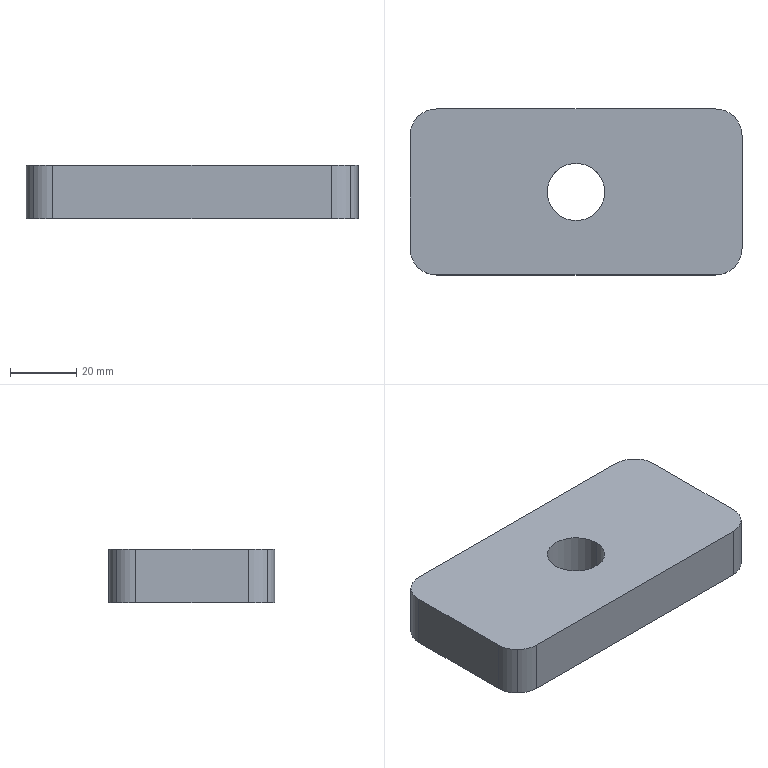Part | STEP file | DCV-000-025 | 1 solid | 16 faces | box 100 x 50 x 16 mm | volume 75363 mm3 | cylinder 10 | plane 6 | commonest cylinder face diameters 16 x8 17.294 x2
STEP:
#1=CARTESIAN_POINT('',(0.,0.,0.));
#2=DIRECTION('',(0.,0.,1.));
#3=DIRECTION('',(1.,0.,0.));
#4=AXIS2_PLACEMENT_3D('',#1,#2,#3);
#5=CARTESIAN_POINT('',(-50.,-17.,0.));
#6=VERTEX_POINT('',#5);
#7=CARTESIAN_POINT('',(-47.657,-22.657,0.));
#8=VERTEX_POINT('',#7);
#9=CARTESIAN_POINT('',(-42.,-17.,0.));
#10=DIRECTION('',(0.,0.,1.));
#11=DIRECTION('',(-0.7071,-0.7071,0.));
#12=AXIS2_PLACEMENT_3D('',#9,#10,#11);
#13=CIRCLE('',#12,8.);
#14=CARTESIAN_POINT('',(-42.,-17.,0.));
#15=DIRECTION('',(0.,0.,1.));
#16=DIRECTION('',(-0.7071,-0.7071,0.));
#17=AXIS2_PLACEMENT_3D('',#14,#15,#16);
#18=CYLINDRICAL_SURFACE('',#17,8.);
#19=CARTESIAN_POINT('',(0.,0.));
#20=DIRECTION('',(1.,0.));
#21=VECTOR('',#20,1.);
#22=LINE('',#19,#21);
#23=(GEOMETRIC_REPRESENTATION_CONTEXT(2)PARAMETRIC_REPRESENTATION_CONTEXT()REPRESENTATION_CONTEXT('',''));
#24=DEFINITIONAL_REPRESENTATION('',(#22),#23);
#25=PCURVE('',#18,#24);
#26=CARTESIAN_POINT('',(0.,0.,0.));
#27=DIRECTION('',(0.,0.,1.));
#28=DIRECTION('',(1.,0.,0.));
#29=AXIS2_PLACEMENT_3D('',#26,#27,#28);
#30=PLANE('',#29);
#31=CARTESIAN_POINT('',(-42.,-17.));
#32=DIRECTION('',(-0.7071,-0.7071));
#33=AXIS2_PLACEMENT_2D('',#31,#32);
#34=CIRCLE('',#33,8.);
#35=(GEOMETRIC_REPRESENTATION_CONTEXT(2)PARAMETRIC_REPRESENTATION_CONTEXT()REPRESENTATION_CONTEXT('',''));
#36=DEFINITIONAL_REPRESENTATION('',(#34),#35);
#37=PCURVE('',#30,#36);
#38=SURFACE_CURVE('',#13,(#25,#37),.PCURVE_S1.);
#39=EDGE_CURVE('',#6,#8,#38,.T.);
#40=ORIENTED_EDGE('',*,*,#39,.T.);
#41=CARTESIAN_POINT('',(-47.657,-22.657,16.));
#42=VERTEX_POINT('',#41);
#43=CARTESIAN_POINT('',(-47.657,-22.657,0.));
#44=DIRECTION('',(0.,0.,1.));
#45=VECTOR('',#44,1.);
#46=LINE('',#43,#45);
#47=CARTESIAN_POINT('',(6.283,0.));
#48=DIRECTION('',(0.,1.));
#49=VECTOR('',#48,1.);
#50=LINE('',#47,#49);
#51=(GEOMETRIC_REPRESENTATION_CONTEXT(2)PARAMETRIC_REPRESENTATION_CONTEXT()REPRESENTATION_CONTEXT('',''));
#52=DEFINITIONAL_REPRESENTATION('',(#50),#51);
#53=PCURVE('',#18,#52);
#54=CARTESIAN_POINT('',(-42.,-17.,0.));
#55=DIRECTION('',(0.,0.,1.));
#56=DIRECTION('',(-0.7071,-0.7071,0.));
#57=AXIS2_PLACEMENT_3D('',#54,#55,#56);
#58=CYLINDRICAL_SURFACE('',#57,8.);
#59=CARTESIAN_POINT('',(0.,0.));
#60=DIRECTION('',(0.,1.));
#61=VECTOR('',#60,1.);
#62=LINE('',#59,#61);
#63=(GEOMETRIC_REPRESENTATION_CONTEXT(2)PARAMETRIC_REPRESENTATION_CONTEXT()REPRESENTATION_CONTEXT('',''));
#64=DEFINITIONAL_REPRESENTATION('',(#62),#63);
#65=PCURVE('',#58,#64);
#66=SURFACE_CURVE('',#46,(#53,#65),.PCURVE_S1.);
#67=EDGE_CURVE('',#8,#42,#66,.T.);
#68=ORIENTED_EDGE('',*,*,#67,.T.);
#69=CARTESIAN_POINT('',(-50.,-17.,16.));
#70=VERTEX_POINT('',#69);
#71=CARTESIAN_POINT('',(-42.,-17.,16.));
#72=DIRECTION('',(0.,0.,-1.));
#73=DIRECTION('',(-0.7071,-0.7071,0.));
#74=AXIS2_PLACEMENT_3D('',#71,#72,#73);
#75=CIRCLE('',#74,8.);
#76=CARTESIAN_POINT('',(6.283,16.));
#77=DIRECTION('',(-1.,0.));
#78=VECTOR('',#77,1.);
#79=LINE('',#76,#78);
#80=(GEOMETRIC_REPRESENTATION_CONTEXT(2)PARAMETRIC_REPRESENTATION_CONTEXT()REPRESENTATION_CONTEXT('',''));
#81=DEFINITIONAL_REPRESENTATION('',(#79),#80);
#82=PCURVE('',#18,#81);
#83=CARTESIAN_POINT('',(0.,0.,16.));
#84=DIRECTION('',(0.,0.,1.));
#85=DIRECTION('',(1.,0.,0.));
#86=AXIS2_PLACEMENT_3D('',#83,#84,#85);
#87=PLANE('',#86);
#88=CARTESIAN_POINT('',(-47.657,-22.657));
#89=CARTESIAN_POINT('',(-57.455,-12.859));
#90=CARTESIAN_POINT('',(-44.071,-9.273));
#91=CARTESIAN_POINT('',(-30.686,-5.686));
#92=CARTESIAN_POINT('',(-34.273,-19.071));
#93=CARTESIAN_POINT('',(-37.859,-32.455));
#94=CARTESIAN_POINT('',(-47.657,-22.657));
#95=(BOUNDED_CURVE()B_SPLINE_CURVE(2,(#88,#89,#90,#91,#92,#93,#94),.UNSPECIFIED.,.T.,.F.)B_SPLINE_CURVE_WITH_KNOTS((1,2,2,2,2,1),(-2.094,0.,2.094,4.189,6.283,8.378),.UNSPECIFIED.)CURVE()GEOMETRIC_REPRESENTATION_ITEM()RATIONAL_B_SPLINE_CURVE((1.,0.5,1.,0.5,1.,0.5,1.))REPRESENTATION_ITEM(''));
#96=(GEOMETRIC_REPRESENTATION_CONTEXT(2)PARAMETRIC_REPRESENTATION_CONTEXT()REPRESENTATION_CONTEXT('',''));
#97=DEFINITIONAL_REPRESENTATION('',(#95),#96);
#98=PCURVE('',#87,#97);
#99=SURFACE_CURVE('',#75,(#82,#98),.PCURVE_S1.);
#100=EDGE_CURVE('',#42,#70,#99,.T.);
#101=ORIENTED_EDGE('',*,*,#100,.T.);
#102=CARTESIAN_POINT('',(-50.,-17.,0.));
#103=DIRECTION('',(0.,0.,-1.));
#104=VECTOR('',#103,1.);
#105=LINE('',#102,#104);
#106=CARTESIAN_POINT('',(5.498,0.));
#107=DIRECTION('',(0.,-1.));
#108=VECTOR('',#107,1.);
#109=LINE('',#106,#108);
#110=(GEOMETRIC_REPRESENTATION_CONTEXT(2)PARAMETRIC_REPRESENTATION_CONTEXT()REPRESENTATION_CONTEXT('',''));
#111=DEFINITIONAL_REPRESENTATION('',(#109),#110);
#112=PCURVE('',#18,#111);
#113=CARTESIAN_POINT('',(-50.,25.,0.));
#114=DIRECTION('',(-1.,0.,0.));
#115=DIRECTION('',(0.,0.,1.));
#116=AXIS2_PLACEMENT_3D('',#113,#114,#115);
#117=PLANE('',#116);
#118=CARTESIAN_POINT('',(0.,-42.));
#119=DIRECTION('',(-1.,0.));
#120=VECTOR('',#119,1.);
#121=LINE('',#118,#120);
#122=(GEOMETRIC_REPRESENTATION_CONTEXT(2)PARAMETRIC_REPRESENTATION_CONTEXT()REPRESENTATION_CONTEXT('',''));
#123=DEFINITIONAL_REPRESENTATION('',(#121),#122);
#124=PCURVE('',#117,#123);
#125=SURFACE_CURVE('',#105,(#112,#124),.PCURVE_S1.);
#126=EDGE_CURVE('',#70,#6,#125,.T.);
#127=ORIENTED_EDGE('',*,*,#126,.T.);
#128=EDGE_LOOP('',(#40,#68,#101,#127));
#129=FACE_BOUND('',#128,.T.);
#130=ADVANCED_FACE('',(#129),#18,.T.);
#131=CARTESIAN_POINT('',(42.,-25.,0.));
#132=VERTEX_POINT('',#131);
#133=CARTESIAN_POINT('',(47.657,-22.657,0.));
#134=VERTEX_POINT('',#133);
#135=CARTESIAN_POINT('',(42.,-17.,0.));
#136=DIRECTION('',(0.,0.,1.));
#137=DIRECTION('',(0.7071,-0.7071,0.));
#138=AXIS2_PLACEMENT_3D('',#135,#136,#137);
#139=CIRCLE('',#138,8.);
#140=CARTESIAN_POINT('',(42.,-17.,0.));
#141=DIRECTION('',(0.,0.,1.));
#142=DIRECTION('',(0.7071,-0.7071,0.));
#143=AXIS2_PLACEMENT_3D('',#140,#141,#142);
#144=CYLINDRICAL_SURFACE('',#143,8.);
#145=CARTESIAN_POINT('',(0.,0.));
#146=DIRECTION('',(1.,0.));
#147=VECTOR('',#146,1.);
#148=LINE('',#145,#147);
#149=(GEOMETRIC_REPRESENTATION_CONTEXT(2)PARAMETRIC_REPRESENTATION_CONTEXT()REPRESENTATION_CONTEXT('',''));
#150=DEFINITIONAL_REPRESENTATION('',(#148),#149);
#151=PCURVE('',#144,#150);
#152=CARTESIAN_POINT('',(42.,-17.));
#153=DIRECTION('',(0.7071,-0.7071));
#154=AXIS2_PLACEMENT_2D('',#152,#153);
#155=CIRCLE('',#154,8.);
#156=(GEOMETRIC_REPRESENTATION_CONTEXT(2)PARAMETRIC_REPRESENTATION_CONTEXT()REPRESENTATION_CONTEXT('',''));
#157=DEFINITIONAL_REPRESENTATION('',(#155),#156);
#158=PCURVE('',#30,#157);
#159=SURFACE_CURVE('',#139,(#151,#158),.PCURVE_S1.);
#160=EDGE_CURVE('',#132,#134,#159,.T.);
#161=ORIENTED_EDGE('',*,*,#160,.T.);
#162=CARTESIAN_POINT('',(47.657,-22.657,16.));
#163=VERTEX_POINT('',#162);
#164=CARTESIAN_POINT('',(47.657,-22.657,0.));
#165=DIRECTION('',(0.,0.,1.));
#166=VECTOR('',#165,1.);
#167=LINE('',#164,#166);
#168=CARTESIAN_POINT('',(6.283,0.));
#169=DIRECTION('',(0.,1.));
#170=VECTOR('',#169,1.);
#171=LINE('',#168,#170);
#172=(GEOMETRIC_REPRESENTATION_CONTEXT(2)PARAMETRIC_REPRESENTATION_CONTEXT()REPRESENTATION_CONTEXT('',''));
#173=DEFINITIONAL_REPRESENTATION('',(#171),#172);
#174=PCURVE('',#144,#173);
#175=CARTESIAN_POINT('',(42.,-17.,0.));
#176=DIRECTION('',(0.,0.,1.));
#177=DIRECTION('',(0.7071,-0.7071,0.));
#178=AXIS2_PLACEMENT_3D('',#175,#176,#177);
#179=CYLINDRICAL_SURFACE('',#178,8.);
#180=CARTESIAN_POINT('',(0.,0.));
#181=DIRECTION('',(0.,1.));
#182=VECTOR('',#181,1.);
#183=LINE('',#180,#182);
#184=(GEOMETRIC_REPRESENTATION_CONTEXT(2)PARAMETRIC_REPRESENTATION_CONTEXT()REPRESENTATION_CONTEXT('',''));
#185=DEFINITIONAL_REPRESENTATION('',(#183),#184);
#186=PCURVE('',#179,#185);
#187=SURFACE_CURVE('',#167,(#174,#186),.PCURVE_S1.);
#188=EDGE_CURVE('',#134,#163,#187,.T.);
#189=ORIENTED_EDGE('',*,*,#188,.T.);
#190=CARTESIAN_POINT('',(42.,-25.,16.));
#191=VERTEX_POINT('',#190);
#192=CARTESIAN_POINT('',(42.,-17.,16.));
#193=DIRECTION('',(0.,0.,-1.));
#194=DIRECTION('',(0.7071,-0.7071,0.));
#195=AXIS2_PLACEMENT_3D('',#192,#193,#194);
#196=CIRCLE('',#195,8.);
#197=CARTESIAN_POINT('',(6.283,16.));
#198=DIRECTION('',(-1.,0.));
#199=VECTOR('',#198,1.);
#200=LINE('',#197,#199);
#201=(GEOMETRIC_REPRESENTATION_CONTEXT(2)PARAMETRIC_REPRESENTATION_CONTEXT()REPRESENTATION_CONTEXT('',''));
#202=DEFINITIONAL_REPRESENTATION('',(#200),#201);
#203=PCURVE('',#144,#202);
#204=CARTESIAN_POINT('',(47.657,-22.657));
#205=CARTESIAN_POINT('',(37.859,-32.455));
#206=CARTESIAN_POINT('',(34.273,-19.071));
#207=CARTESIAN_POINT('',(30.686,-5.686));
#208=CARTESIAN_POINT('',(44.071,-9.273));
#209=CARTESIAN_POINT('',(57.455,-12.859));
#210=CARTESIAN_POINT('',(47.657,-22.657));
#211=(BOUNDED_CURVE()B_SPLINE_CURVE(2,(#204,#205,#206,#207,#208,#209,#210),.UNSPECIFIED.,.T.,.F.)B_SPLINE_CURVE_WITH_KNOTS((1,2,2,2,2,1),(-2.094,0.,2.094,4.189,6.283,8.378),.UNSPECIFIED.)CURVE()GEOMETRIC_REPRESENTATION_ITEM()RATIONAL_B_SPLINE_CURVE((1.,0.5,1.,0.5,1.,0.5,1.))REPRESENTATION_ITEM(''));
#212=(GEOMETRIC_REPRESENTATION_CONTEXT(2)PARAMETRIC_REPRESENTATION_CONTEXT()REPRESENTATION_CONTEXT('',''));
#213=DEFINITIONAL_REPRESENTATION('',(#211),#212);
#214=PCURVE('',#87,#213);
#215=SURFACE_CURVE('',#196,(#203,#214),.PCURVE_S1.);
#216=EDGE_CURVE('',#163,#191,#215,.T.);
#217=ORIENTED_EDGE('',*,*,#216,.T.);
#218=CARTESIAN_POINT('',(42.,-25.,0.));
#219=DIRECTION('',(0.,0.,-1.));
#220=VECTOR('',#219,1.);
#221=LINE('',#218,#220);
#222=CARTESIAN_POINT('',(5.498,0.));
#223=DIRECTION('',(0.,-1.));
#224=VECTOR('',#223,1.);
#225=LINE('',#222,#224);
#226=(GEOMETRIC_REPRESENTATION_CONTEXT(2)PARAMETRIC_REPRESENTATION_CONTEXT()REPRESENTATION_CONTEXT('',''));
#227=DEFINITIONAL_REPRESENTATION('',(#225),#226);
#228=PCURVE('',#144,#227);
#229=CARTESIAN_POINT('',(-50.,-25.,0.));
#230=DIRECTION('',(0.,-1.,0.));
#231=DIRECTION('',(0.,0.,-1.));
#232=AXIS2_PLACEMENT_3D('',#229,#230,#231);
#233=PLANE('',#232);
#234=CARTESIAN_POINT('',(0.,92.));
#235=DIRECTION('',(1.,0.));
#236=VECTOR('',#235,1.);
#237=LINE('',#234,#236);
#238=(GEOMETRIC_REPRESENTATION_CONTEXT(2)PARAMETRIC_REPRESENTATION_CONTEXT()REPRESENTATION_CONTEXT('',''));
#239=DEFINITIONAL_REPRESENTATION('',(#237),#238);
#240=PCURVE('',#233,#239);
#241=SURFACE_CURVE('',#221,(#228,#240),.PCURVE_S1.);
#242=EDGE_CURVE('',#191,#132,#241,.T.);
#243=ORIENTED_EDGE('',*,*,#242,.T.);
#244=EDGE_LOOP('',(#161,#189,#217,#243));
#245=FACE_BOUND('',#244,.T.);
#246=ADVANCED_FACE('',(#245),#144,.T.);
#247=CARTESIAN_POINT('',(50.,17.,0.));
#248=VERTEX_POINT('',#247);
#249=CARTESIAN_POINT('',(47.657,22.657,0.));
#250=VERTEX_POINT('',#249);
#251=CARTESIAN_POINT('',(42.,17.,0.));
#252=DIRECTION('',(0.,0.,1.));
#253=DIRECTION('',(0.7071,0.7071,0.));
#254=AXIS2_PLACEMENT_3D('',#251,#252,#253);
#255=CIRCLE('',#254,8.);
#256=CARTESIAN_POINT('',(42.,17.,0.));
#257=DIRECTION('',(0.,0.,1.));
#258=DIRECTION('',(0.7071,0.7071,0.));
#259=AXIS2_PLACEMENT_3D('',#256,#257,#258);
#260=CYLINDRICAL_SURFACE('',#259,8.);
#261=CARTESIAN_POINT('',(0.,0.));
#262=DIRECTION('',(1.,0.));
#263=VECTOR('',#262,1.);
#264=LINE('',#261,#263);
#265=(GEOMETRIC_REPRESENTATION_CONTEXT(2)PARAMETRIC_REPRESENTATION_CONTEXT()REPRESENTATION_CONTEXT('',''));
#266=DEFINITIONAL_REPRESENTATION('',(#264),#265);
#267=PCURVE('',#260,#266);
#268=CARTESIAN_POINT('',(42.,17.));
#269=DIRECTION('',(0.7071,0.7071));
#270=AXIS2_PLACEMENT_2D('',#268,#269);
#271=CIRCLE('',#270,8.);
#272=(GEOMETRIC_REPRESENTATION_CONTEXT(2)PARAMETRIC_REPRESENTATION_CONTEXT()REPRESENTATION_CONTEXT('',''));
#273=DEFINITIONAL_REPRESENTATION('',(#271),#272);
#274=PCURVE('',#30,#273);
#275=SURFACE_CURVE('',#255,(#267,#274),.PCURVE_S1.);
#276=EDGE_CURVE('',#248,#250,#275,.T.);
#277=ORIENTED_EDGE('',*,*,#276,.T.);
#278=CARTESIAN_POINT('',(47.657,22.657,16.));
#279=VERTEX_POINT('',#278);
#280=CARTESIAN_POINT('',(47.657,22.657,0.));
#281=DIRECTION('',(0.,0.,1.));
#282=VECTOR('',#281,1.);
#283=LINE('',#280,#282);
#284=CARTESIAN_POINT('',(6.283,0.));
#285=DIRECTION('',(0.,1.));
#286=VECTOR('',#285,1.);
#287=LINE('',#284,#286);
#288=(GEOMETRIC_REPRESENTATION_CONTEXT(2)PARAMETRIC_REPRESENTATION_CONTEXT()REPRESENTATION_CONTEXT('',''));
#289=DEFINITIONAL_REPRESENTATION('',(#287),#288);
#290=PCURVE('',#260,#289);
#291=CARTESIAN_POINT('',(42.,17.,0.));
#292=DIRECTION('',(0.,0.,1.));
#293=DIRECTION('',(0.7071,0.7071,0.));
#294=AXIS2_PLACEMENT_3D('',#291,#292,#293);
#295=CYLINDRICAL_SURFACE('',#294,8.);
#296=CARTESIAN_POINT('',(0.,0.));
#297=DIRECTION('',(0.,1.));
#298=VECTOR('',#297,1.);
#299=LINE('',#296,#298);
#300=(GEOMETRIC_REPRESENTATION_CONTEXT(2)PARAMETRIC_REPRESENTATION_CONTEXT()REPRESENTATION_CONTEXT('',''));
#301=DEFINITIONAL_REPRESENTATION('',(#299),#300);
#302=PCURVE('',#295,#301);
#303=SURFACE_CURVE('',#283,(#290,#302),.PCURVE_S1.);
#304=EDGE_CURVE('',#250,#279,#303,.T.);
#305=ORIENTED_EDGE('',*,*,#304,.T.);
#306=CARTESIAN_POINT('',(50.,17.,16.));
#307=VERTEX_POINT('',#306);
#308=CARTESIAN_POINT('',(42.,17.,16.));
#309=DIRECTION('',(0.,0.,-1.));
#310=DIRECTION('',(0.7071,0.7071,0.));
#311=AXIS2_PLACEMENT_3D('',#308,#309,#310);
#312=CIRCLE('',#311,8.);
#313=CARTESIAN_POINT('',(6.283,16.));
#314=DIRECTION('',(-1.,0.));
#315=VECTOR('',#314,1.);
#316=LINE('',#313,#315);
#317=(GEOMETRIC_REPRESENTATION_CONTEXT(2)PARAMETRIC_REPRESENTATION_CONTEXT()REPRESENTATION_CONTEXT('',''));
#318=DEFINITIONAL_REPRESENTATION('',(#316),#317);
#319=PCURVE('',#260,#318);
#320=CARTESIAN_POINT('',(47.657,22.657));
#321=CARTESIAN_POINT('',(57.455,12.859));
#322=CARTESIAN_POINT('',(44.071,9.273));
#323=CARTESIAN_POINT('',(30.686,5.686));
#324=CARTESIAN_POINT('',(34.273,19.071));
#325=CARTESIAN_POINT('',(37.859,32.455));
#326=CARTESIAN_POINT('',(47.657,22.657));
#327=(BOUNDED_CURVE()B_SPLINE_CURVE(2,(#320,#321,#322,#323,#324,#325,#326),.UNSPECIFIED.,.T.,.F.)B_SPLINE_CURVE_WITH_KNOTS((1,2,2,2,2,1),(-2.094,0.,2.094,4.189,6.283,8.378),.UNSPECIFIED.)CURVE()GEOMETRIC_REPRESENTATION_ITEM()RATIONAL_B_SPLINE_CURVE((1.,0.5,1.,0.5,1.,0.5,1.))REPRESENTATION_ITEM(''));
#328=(GEOMETRIC_REPRESENTATION_CONTEXT(2)PARAMETRIC_REPRESENTATION_CONTEXT()REPRESENTATION_CONTEXT('',''));
#329=DEFINITIONAL_REPRESENTATION('',(#327),#328);
#330=PCURVE('',#87,#329);
#331=SURFACE_CURVE('',#312,(#319,#330),.PCURVE_S1.);
#332=EDGE_CURVE('',#279,#307,#331,.T.);
#333=ORIENTED_EDGE('',*,*,#332,.T.);
#334=CARTESIAN_POINT('',(50.,17.,0.));
#335=DIRECTION('',(0.,0.,-1.));
#336=VECTOR('',#335,1.);
#337=LINE('',#334,#336);
#338=CARTESIAN_POINT('',(5.498,0.));
#339=DIRECTION('',(0.,-1.));
#340=VECTOR('',#339,1.);
#341=LINE('',#338,#340);
#342=(GEOMETRIC_REPRESENTATION_CONTEXT(2)PARAMETRIC_REPRESENTATION_CONTEXT()REPRESENTATION_CONTEXT('',''));
#343=DEFINITIONAL_REPRESENTATION('',(#341),#342);
#344=PCURVE('',#260,#343);
#345=CARTESIAN_POINT('',(50.,-25.,0.));
#346=DIRECTION('',(1.,0.,0.));
#347=DIRECTION('',(0.,1.,0.));
#348=AXIS2_PLACEMENT_3D('',#345,#346,#347);
#349=PLANE('',#348);
#350=CARTESIAN_POINT('',(42.,0.));
#351=DIRECTION('',(0.,-1.));
#352=VECTOR('',#351,1.);
#353=LINE('',#350,#352);
#354=(GEOMETRIC_REPRESENTATION_CONTEXT(2)PARAMETRIC_REPRESENTATION_CONTEXT()REPRESENTATION_CONTEXT('',''));
#355=DEFINITIONAL_REPRESENTATION('',(#353),#354);
#356=PCURVE('',#349,#355);
#357=SURFACE_CURVE('',#337,(#344,#356),.PCURVE_S1.);
#358=EDGE_CURVE('',#307,#248,#357,.T.);
#359=ORIENTED_EDGE('',*,*,#358,.T.);
#360=EDGE_LOOP('',(#277,#305,#333,#359));
#361=FACE_BOUND('',#360,.T.);
#362=ADVANCED_FACE('',(#361),#260,.T.);
#363=CARTESIAN_POINT('',(-42.,25.,0.));
#364=VERTEX_POINT('',#363);
#365=CARTESIAN_POINT('',(-47.657,22.657,0.));
#366=VERTEX_POINT('',#365);
#367=CARTESIAN_POINT('',(-42.,17.,0.));
#368=DIRECTION('',(0.,0.,1.));
#369=DIRECTION('',(-0.7071,0.7071,0.));
#370=AXIS2_PLACEMENT_3D('',#367,#368,#369);
#371=CIRCLE('',#370,8.);
#372=CARTESIAN_POINT('',(-42.,17.,0.));
#373=DIRECTION('',(0.,0.,1.));
#374=DIRECTION('',(-0.7071,0.7071,0.));
#375=AXIS2_PLACEMENT_3D('',#372,#373,#374);
#376=CYLINDRICAL_SURFACE('',#375,8.);
#377=CARTESIAN_POINT('',(0.,0.));
#378=DIRECTION('',(1.,0.));
#379=VECTOR('',#378,1.);
#380=LINE('',#377,#379);
#381=(GEOMETRIC_REPRESENTATION_CONTEXT(2)PARAMETRIC_REPRESENTATION_CONTEXT()REPRESENTATION_CONTEXT('',''));
#382=DEFINITIONAL_REPRESENTATION('',(#380),#381);
#383=PCURVE('',#376,#382);
#384=CARTESIAN_POINT('',(-42.,17.));
#385=DIRECTION('',(-0.7071,0.7071));
#386=AXIS2_PLACEMENT_2D('',#384,#385);
#387=CIRCLE('',#386,8.);
#388=(GEOMETRIC_REPRESENTATION_CONTEXT(2)PARAMETRIC_REPRESENTATION_CONTEXT()REPRESENTATION_CONTEXT('',''));
#389=DEFINITIONAL_REPRESENTATION('',(#387),#388);
#390=PCURVE('',#30,#389);
#391=SURFACE_CURVE('',#371,(#383,#390),.PCURVE_S1.);
#392=EDGE_CURVE('',#364,#366,#391,.T.);
#393=ORIENTED_EDGE('',*,*,#392,.T.);
#394=CARTESIAN_POINT('',(-47.657,22.657,16.));
#395=VERTEX_POINT('',#394);
#396=CARTESIAN_POINT('',(-47.657,22.657,0.));
#397=DIRECTION('',(0.,0.,1.));
#398=VECTOR('',#397,1.);
#399=LINE('',#396,#398);
#400=CARTESIAN_POINT('',(6.283,0.));
#401=DIRECTION('',(0.,1.));
#402=VECTOR('',#401,1.);
#403=LINE('',#400,#402);
#404=(GEOMETRIC_REPRESENTATION_CONTEXT(2)PARAMETRIC_REPRESENTATION_CONTEXT()REPRESENTATION_CONTEXT('',''));
#405=DEFINITIONAL_REPRESENTATION('',(#403),#404);
#406=PCURVE('',#376,#405);
#407=CARTESIAN_POINT('',(-42.,17.,0.));
#408=DIRECTION('',(0.,0.,1.));
#409=DIRECTION('',(-0.7071,0.7071,0.));
#410=AXIS2_PLACEMENT_3D('',#407,#408,#409);
#411=CYLINDRICAL_SURFACE('',#410,8.);
#412=CARTESIAN_POINT('',(0.,0.));
#413=DIRECTION('',(0.,1.));
#414=VECTOR('',#413,1.);
#415=LINE('',#412,#414);
#416=(GEOMETRIC_REPRESENTATION_CONTEXT(2)PARAMETRIC_REPRESENTATION_CONTEXT()REPRESENTATION_CONTEXT('',''));
#417=DEFINITIONAL_REPRESENTATION('',(#415),#416);
#418=PCURVE('',#411,#417);
#419=SURFACE_CURVE('',#399,(#406,#418),.PCURVE_S1.);
#420=EDGE_CURVE('',#366,#395,#419,.T.);
#421=ORIENTED_EDGE('',*,*,#420,.T.);
#422=CARTESIAN_POINT('',(-42.,25.,16.));
#423=VERTEX_POINT('',#422);
#424=CARTESIAN_POINT('',(-42.,17.,16.));
#425=DIRECTION('',(0.,0.,-1.));
#426=DIRECTION('',(-0.7071,0.7071,0.));
#427=AXIS2_PLACEMENT_3D('',#424,#425,#426);
#428=CIRCLE('',#427,8.);
#429=CARTESIAN_POINT('',(6.283,16.));
#430=DIRECTION('',(-1.,0.));
#431=VECTOR('',#430,1.);
#432=LINE('',#429,#431);
#433=(GEOMETRIC_REPRESENTATION_CONTEXT(2)PARAMETRIC_REPRESENTATION_CONTEXT()REPRESENTATION_CONTEXT('',''));
#434=DEFINITIONAL_REPRESENTATION('',(#432),#433);
#435=PCURVE('',#376,#434);
#436=CARTESIAN_POINT('',(-47.657,22.657));
#437=CARTESIAN_POINT('',(-37.859,32.455));
#438=CARTESIAN_POINT('',(-34.273,19.071));
#439=CARTESIAN_POINT('',(-30.686,5.686));
#440=CARTESIAN_POINT('',(-44.071,9.273));
#441=CARTESIAN_POINT('',(-57.455,12.859));
#442=CARTESIAN_POINT('',(-47.657,22.657));
#443=(BOUNDED_CURVE()B_SPLINE_CURVE(2,(#436,#437,#438,#439,#440,#441,#442),.UNSPECIFIED.,.T.,.F.)B_SPLINE_CURVE_WITH_KNOTS((1,2,2,2,2,1),(-2.094,0.,2.094,4.189,6.283,8.378),.UNSPECIFIED.)CURVE()GEOMETRIC_REPRESENTATION_ITEM()RATIONAL_B_SPLINE_CURVE((1.,0.5,1.,0.5,1.,0.5,1.))REPRESENTATION_ITEM(''));
#444=(GEOMETRIC_REPRESENTATION_CONTEXT(2)PARAMETRIC_REPRESENTATION_CONTEXT()REPRESENTATION_CONTEXT('',''));
#445=DEFINITIONAL_REPRESENTATION('',(#443),#444);
#446=PCURVE('',#87,#445);
#447=SURFACE_CURVE('',#428,(#435,#446),.PCURVE_S1.);
#448=EDGE_CURVE('',#395,#423,#447,.T.);
#449=ORIENTED_EDGE('',*,*,#448,.T.);
#450=CARTESIAN_POINT('',(-42.,25.,0.));
#451=DIRECTION('',(0.,0.,-1.));
#452=VECTOR('',#451,1.);
#453=LINE('',#450,#452);
#454=CARTESIAN_POINT('',(5.498,0.));
#455=DIRECTION('',(0.,-1.));
#456=VECTOR('',#455,1.);
#457=LINE('',#454,#456);
#458=(GEOMETRIC_REPRESENTATION_CONTEXT(2)PARAMETRIC_REPRESENTATION_CONTEXT()REPRESENTATION_CONTEXT('',''));
#459=DEFINITIONAL_REPRESENTATION('',(#457),#458);
#460=PCURVE('',#376,#459);
#461=CARTESIAN_POINT('',(50.,25.,0.));
#462=DIRECTION('',(0.,1.,0.));
#463=DIRECTION('',(1.,0.,0.));
#464=AXIS2_PLACEMENT_3D('',#461,#462,#463);
#465=PLANE('',#464);
#466=CARTESIAN_POINT('',(-92.,0.));
#467=DIRECTION('',(0.,1.));
#468=VECTOR('',#467,1.);
#469=LINE('',#466,#468);
#470=(GEOMETRIC_REPRESENTATION_CONTEXT(2)PARAMETRIC_REPRESENTATION_CONTEXT()REPRESENTATION_CONTEXT('',''));
#471=DEFINITIONAL_REPRESENTATION('',(#469),#470);
#472=PCURVE('',#465,#471);
#473=SURFACE_CURVE('',#453,(#460,#472),.PCURVE_S1.);
#474=EDGE_CURVE('',#423,#364,#473,.T.);
#475=ORIENTED_EDGE('',*,*,#474,.T.);
#476=EDGE_LOOP('',(#393,#421,#449,#475));
#477=FACE_BOUND('',#476,.T.);
#478=ADVANCED_FACE('',(#477),#376,.T.);
#479=CARTESIAN_POINT('',(8.647,0.,0.));
#480=VERTEX_POINT('',#479);
#481=CARTESIAN_POINT('',(8.647,0.,16.));
#482=VERTEX_POINT('',#481);
#483=CARTESIAN_POINT('',(8.647,0.,-96.942));
#484=DIRECTION('',(0.,0.,1.));
#485=VECTOR('',#484,1.);
#486=LINE('',#483,#485);
#487=CARTESIAN_POINT('',(0.,0.,-96.942));
#488=DIRECTION('',(0.,0.,1.));
#489=DIRECTION('',(1.,0.,0.));
#490=AXIS2_PLACEMENT_3D('',#487,#488,#489);
#491=CYLINDRICAL_SURFACE('',#490,8.647);
#492=CARTESIAN_POINT('',(6.283,0.));
#493=DIRECTION('',(0.,1.));
#494=VECTOR('',#493,1.);
#495=LINE('',#492,#494);
#496=(GEOMETRIC_REPRESENTATION_CONTEXT(2)PARAMETRIC_REPRESENTATION_CONTEXT()REPRESENTATION_CONTEXT('',''));
#497=DEFINITIONAL_REPRESENTATION('',(#495),#496);
#498=PCURVE('',#491,#497);
#499=CARTESIAN_POINT('',(0.,0.,-96.942));
#500=DIRECTION('',(0.,0.,1.));
#501=DIRECTION('',(1.,0.,0.));
#502=AXIS2_PLACEMENT_3D('',#499,#500,#501);
#503=CYLINDRICAL_SURFACE('',#502,8.647);
#504=CARTESIAN_POINT('',(0.,0.));
#505=DIRECTION('',(0.,1.));
#506=VECTOR('',#505,1.);
#507=LINE('',#504,#506);
#508=(GEOMETRIC_REPRESENTATION_CONTEXT(2)PARAMETRIC_REPRESENTATION_CONTEXT()REPRESENTATION_CONTEXT('',''));
#509=DEFINITIONAL_REPRESENTATION('',(#507),#508);
#510=PCURVE('',#503,#509);
#511=SURFACE_CURVE('',#486,(#498,#510),.PCURVE_S1.);
#512=EDGE_CURVE('',#480,#482,#511,.T.);
#513=ORIENTED_EDGE('',*,*,#512,.T.);
#514=CARTESIAN_POINT('',(-8.647,0.,16.));
#515=VERTEX_POINT('',#514);
#516=CARTESIAN_POINT('',(0.,0.,16.));
#517=DIRECTION('',(0.,0.,-1.));
#518=DIRECTION('',(1.,0.,0.));
#519=AXIS2_PLACEMENT_3D('',#516,#517,#518);
#520=CIRCLE('',#519,8.647);
#521=CARTESIAN_POINT('',(6.283,112.942));
#522=DIRECTION('',(-1.,0.));
#523=VECTOR('',#522,1.);
#524=LINE('',#521,#523);
#525=(GEOMETRIC_REPRESENTATION_CONTEXT(2)PARAMETRIC_REPRESENTATION_CONTEXT()REPRESENTATION_CONTEXT('',''));
#526=DEFINITIONAL_REPRESENTATION('',(#524),#525);
#527=PCURVE('',#491,#526);
#528=CARTESIAN_POINT('',(8.647,0.));
#529=CARTESIAN_POINT('',(8.647,-14.977));
#530=CARTESIAN_POINT('',(-4.324,-7.489));
#531=CARTESIAN_POINT('',(-17.294,0.));
#532=CARTESIAN_POINT('',(-4.324,7.489));
#533=CARTESIAN_POINT('',(8.647,14.977));
#534=CARTESIAN_POINT('',(8.647,0.));
#535=(BOUNDED_CURVE()B_SPLINE_CURVE(2,(#528,#529,#530,#531,#532,#533,#534),.UNSPECIFIED.,.T.,.F.)B_SPLINE_CURVE_WITH_KNOTS((1,2,2,2,2,1),(-2.094,0.,2.094,4.189,6.283,8.378),.UNSPECIFIED.)CURVE()GEOMETRIC_REPRESENTATION_ITEM()RATIONAL_B_SPLINE_CURVE((1.,0.5,1.,0.5,1.,0.5,1.))REPRESENTATION_ITEM(''));
#536=(GEOMETRIC_REPRESENTATION_CONTEXT(2)PARAMETRIC_REPRESENTATION_CONTEXT()REPRESENTATION_CONTEXT('',''));
#537=DEFINITIONAL_REPRESENTATION('',(#535),#536);
#538=PCURVE('',#87,#537);
#539=SURFACE_CURVE('',#520,(#527,#538),.PCURVE_S1.);
#540=EDGE_CURVE('',#482,#515,#539,.T.);
#541=ORIENTED_EDGE('',*,*,#540,.T.);
#542=CARTESIAN_POINT('',(-8.647,0.,0.));
#543=VERTEX_POINT('',#542);
#544=CARTESIAN_POINT('',(-8.647,0.,-96.942));
#545=DIRECTION('',(0.,0.,1.));
#546=VECTOR('',#545,1.);
#547=LINE('',#544,#546);
#548=CARTESIAN_POINT('',(3.142,0.));
#549=DIRECTION('',(0.,1.));
#550=VECTOR('',#549,1.);
#551=LINE('',#548,#550);
#552=(GEOMETRIC_REPRESENTATION_CONTEXT(2)PARAMETRIC_REPRESENTATION_CONTEXT()REPRESENTATION_CONTEXT('',''));
#553=DEFINITIONAL_REPRESENTATION('',(#551),#552);
#554=PCURVE('',#491,#553);
#555=CARTESIAN_POINT('',(3.142,0.));
#556=DIRECTION('',(0.,1.));
#557=VECTOR('',#556,1.);
#558=LINE('',#555,#557);
#559=(GEOMETRIC_REPRESENTATION_CONTEXT(2)PARAMETRIC_REPRESENTATION_CONTEXT()REPRESENTATION_CONTEXT('',''));
#560=DEFINITIONAL_REPRESENTATION('',(#558),#559);
#561=PCURVE('',#503,#560);
#562=SURFACE_CURVE('',#547,(#554,#561),.PCURVE_S1.);
#563=EDGE_CURVE('',#543,#515,#562,.T.);
#564=ORIENTED_EDGE('',*,*,#563,.F.);
#565=CARTESIAN_POINT('',(0.,0.,0.));
#566=DIRECTION('',(0.,0.,1.));
#567=DIRECTION('',(1.,0.,0.));
#568=AXIS2_PLACEMENT_3D('',#565,#566,#567);
#569=CIRCLE('',#568,8.647);
#570=CARTESIAN_POINT('',(0.,96.942));
#571=DIRECTION('',(1.,0.));
#572=VECTOR('',#571,1.);
#573=LINE('',#570,#572);
#574=(GEOMETRIC_REPRESENTATION_CONTEXT(2)PARAMETRIC_REPRESENTATION_CONTEXT()REPRESENTATION_CONTEXT('',''));
#575=DEFINITIONAL_REPRESENTATION('',(#573),#574);
#576=PCURVE('',#491,#575);
#577=CARTESIAN_POINT('',(0.,0.));
#578=DIRECTION('',(1.,0.));
#579=AXIS2_PLACEMENT_2D('',#577,#578);
#580=CIRCLE('',#579,8.647);
#581=(GEOMETRIC_REPRESENTATION_CONTEXT(2)PARAMETRIC_REPRESENTATION_CONTEXT()REPRESENTATION_CONTEXT('',''));
#582=DEFINITIONAL_REPRESENTATION('',(#580),#581);
#583=PCURVE('',#30,#582);
#584=SURFACE_CURVE('',#569,(#576,#583),.PCURVE_S1.);
#585=EDGE_CURVE('',#543,#480,#584,.T.);
#586=ORIENTED_EDGE('',*,*,#585,.T.);
#587=EDGE_LOOP('',(#513,#541,#564,#586));
#588=FACE_BOUND('',#587,.F.);
#589=ADVANCED_FACE('',(#588),#491,.F.);
#590=ORIENTED_EDGE('',*,*,#540,.T.);
#591=CARTESIAN_POINT('',(0.,0.,16.));
#592=DIRECTION('',(0.,0.,-1.));
#593=DIRECTION('',(1.,0.,0.));
#594=AXIS2_PLACEMENT_3D('',#591,#592,#593);
#595=CIRCLE('',#594,8.647);
#596=CARTESIAN_POINT('',(8.647,0.));
#597=CARTESIAN_POINT('',(8.647,-14.977));
#598=CARTESIAN_POINT('',(-4.324,-7.489));
#599=CARTESIAN_POINT('',(-17.294,0.));
#600=CARTESIAN_POINT('',(-4.324,7.489));
#601=CARTESIAN_POINT('',(8.647,14.977));
#602=CARTESIAN_POINT('',(8.647,0.));
#603=(BOUNDED_CURVE()B_SPLINE_CURVE(2,(#596,#597,#598,#599,#600,#601,#602),.UNSPECIFIED.,.T.,.F.)B_SPLINE_CURVE_WITH_KNOTS((1,2,2,2,2,1),(-2.094,0.,2.094,4.189,6.283,8.378),.UNSPECIFIED.)CURVE()GEOMETRIC_REPRESENTATION_ITEM()RATIONAL_B_SPLINE_CURVE((1.,0.5,1.,0.5,1.,0.5,1.))REPRESENTATION_ITEM(''));
#604=(GEOMETRIC_REPRESENTATION_CONTEXT(2)PARAMETRIC_REPRESENTATION_CONTEXT()REPRESENTATION_CONTEXT('',''));
#605=DEFINITIONAL_REPRESENTATION('',(#603),#604);
#606=PCURVE('',#87,#605);
#607=CARTESIAN_POINT('',(6.283,112.942));
#608=DIRECTION('',(-1.,0.));
#609=VECTOR('',#608,1.);
#610=LINE('',#607,#609);
#611=(GEOMETRIC_REPRESENTATION_CONTEXT(2)PARAMETRIC_REPRESENTATION_CONTEXT()REPRESENTATION_CONTEXT('',''));
#612=DEFINITIONAL_REPRESENTATION('',(#610),#611);
#613=PCURVE('',#503,#612);
#614=SURFACE_CURVE('',#595,(#606,#613),.PCURVE_S1.);
#615=EDGE_CURVE('',#515,#482,#614,.T.);
#616=ORIENTED_EDGE('',*,*,#615,.T.);
#617=EDGE_LOOP('',(#590,#616));
#618=FACE_BOUND('',#617,.T.);
#619=CARTESIAN_POINT('',(-42.,-25.,16.));
#620=VERTEX_POINT('',#619);
#621=CARTESIAN_POINT('',(-42.,-17.,16.));
#622=DIRECTION('',(0.,0.,-1.));
#623=DIRECTION('',(-0.7071,-0.7071,0.));
#624=AXIS2_PLACEMENT_3D('',#621,#622,#623);
#625=CIRCLE('',#624,8.);
#626=CARTESIAN_POINT('',(-47.657,-22.657));
#627=CARTESIAN_POINT('',(-57.455,-12.859));
#628=CARTESIAN_POINT('',(-44.071,-9.273));
#629=CARTESIAN_POINT('',(-30.686,-5.686));
#630=CARTESIAN_POINT('',(-34.273,-19.071));
#631=CARTESIAN_POINT('',(-37.859,-32.455));
#632=CARTESIAN_POINT('',(-47.657,-22.657));
#633=(BOUNDED_CURVE()B_SPLINE_CURVE(2,(#626,#627,#628,#629,#630,#631,#632),.UNSPECIFIED.,.T.,.F.)B_SPLINE_CURVE_WITH_KNOTS((1,2,2,2,2,1),(-2.094,0.,2.094,4.189,6.283,8.378),.UNSPECIFIED.)CURVE()GEOMETRIC_REPRESENTATION_ITEM()RATIONAL_B_SPLINE_CURVE((1.,0.5,1.,0.5,1.,0.5,1.))REPRESENTATION_ITEM(''));
#634=(GEOMETRIC_REPRESENTATION_CONTEXT(2)PARAMETRIC_REPRESENTATION_CONTEXT()REPRESENTATION_CONTEXT('',''));
#635=DEFINITIONAL_REPRESENTATION('',(#633),#634);
#636=PCURVE('',#87,#635);
#637=CARTESIAN_POINT('',(6.283,16.));
#638=DIRECTION('',(-1.,0.));
#639=VECTOR('',#638,1.);
#640=LINE('',#637,#639);
#641=(GEOMETRIC_REPRESENTATION_CONTEXT(2)PARAMETRIC_REPRESENTATION_CONTEXT()REPRESENTATION_CONTEXT('',''));
#642=DEFINITIONAL_REPRESENTATION('',(#640),#641);
#643=PCURVE('',#58,#642);
#644=SURFACE_CURVE('',#625,(#636,#643),.PCURVE_S1.);
#645=EDGE_CURVE('',#620,#42,#644,.T.);
#646=ORIENTED_EDGE('',*,*,#645,.F.);
#647=CARTESIAN_POINT('',(-50.,-25.,16.));
#648=DIRECTION('',(1.,0.,0.));
#649=VECTOR('',#648,1.);
#650=LINE('',#647,#649);
#651=CARTESIAN_POINT('',(-50.,-25.));
#652=DIRECTION('',(1.,0.));
#653=VECTOR('',#652,1.);
#654=LINE('',#651,#653);
#655=(GEOMETRIC_REPRESENTATION_CONTEXT(2)PARAMETRIC_REPRESENTATION_CONTEXT()REPRESENTATION_CONTEXT('',''));
#656=DEFINITIONAL_REPRESENTATION('',(#654),#655);
#657=PCURVE('',#87,#656);
#658=CARTESIAN_POINT('',(-16.,0.));
#659=DIRECTION('',(0.,1.));
#660=VECTOR('',#659,1.);
#661=LINE('',#658,#660);
#662=(GEOMETRIC_REPRESENTATION_CONTEXT(2)PARAMETRIC_REPRESENTATION_CONTEXT()REPRESENTATION_CONTEXT('',''));
#663=DEFINITIONAL_REPRESENTATION('',(#661),#662);
#664=PCURVE('',#233,#663);
#665=SURFACE_CURVE('',#650,(#657,#664),.PCURVE_S1.);
#666=EDGE_CURVE('',#620,#191,#665,.T.);
#667=ORIENTED_EDGE('',*,*,#666,.T.);
#668=ORIENTED_EDGE('',*,*,#216,.F.);
#669=CARTESIAN_POINT('',(50.,-17.,16.));
#670=VERTEX_POINT('',#669);
#671=CARTESIAN_POINT('',(42.,-17.,16.));
#672=DIRECTION('',(0.,0.,-1.));
#673=DIRECTION('',(0.7071,-0.7071,0.));
#674=AXIS2_PLACEMENT_3D('',#671,#672,#673);
#675=CIRCLE('',#674,8.);
#676=CARTESIAN_POINT('',(47.657,-22.657));
#677=CARTESIAN_POINT('',(37.859,-32.455));
#678=CARTESIAN_POINT('',(34.273,-19.071));
#679=CARTESIAN_POINT('',(30.686,-5.686));
#680=CARTESIAN_POINT('',(44.071,-9.273));
#681=CARTESIAN_POINT('',(57.455,-12.859));
#682=CARTESIAN_POINT('',(47.657,-22.657));
#683=(BOUNDED_CURVE()B_SPLINE_CURVE(2,(#676,#677,#678,#679,#680,#681,#682),.UNSPECIFIED.,.T.,.F.)B_SPLINE_CURVE_WITH_KNOTS((1,2,2,2,2,1),(-2.094,0.,2.094,4.189,6.283,8.378),.UNSPECIFIED.)CURVE()GEOMETRIC_REPRESENTATION_ITEM()RATIONAL_B_SPLINE_CURVE((1.,0.5,1.,0.5,1.,0.5,1.))REPRESENTATION_ITEM(''));
#684=(GEOMETRIC_REPRESENTATION_CONTEXT(2)PARAMETRIC_REPRESENTATION_CONTEXT()REPRESENTATION_CONTEXT('',''));
#685=DEFINITIONAL_REPRESENTATION('',(#683),#684);
#686=PCURVE('',#87,#685);
#687=CARTESIAN_POINT('',(6.283,16.));
#688=DIRECTION('',(-1.,0.));
#689=VECTOR('',#688,1.);
#690=LINE('',#687,#689);
#691=(GEOMETRIC_REPRESENTATION_CONTEXT(2)PARAMETRIC_REPRESENTATION_CONTEXT()REPRESENTATION_CONTEXT('',''));
#692=DEFINITIONAL_REPRESENTATION('',(#690),#691);
#693=PCURVE('',#179,#692);
#694=SURFACE_CURVE('',#675,(#686,#693),.PCURVE_S1.);
#695=EDGE_CURVE('',#670,#163,#694,.T.);
#696=ORIENTED_EDGE('',*,*,#695,.F.);
#697=CARTESIAN_POINT('',(50.,-25.,16.));
#698=DIRECTION('',(0.,1.,0.));
#699=VECTOR('',#698,1.);
#700=LINE('',#697,#699);
#701=CARTESIAN_POINT('',(50.,-25.));
#702=DIRECTION('',(0.,1.));
#703=VECTOR('',#702,1.);
#704=LINE('',#701,#703);
#705=(GEOMETRIC_REPRESENTATION_CONTEXT(2)PARAMETRIC_REPRESENTATION_CONTEXT()REPRESENTATION_CONTEXT('',''));
#706=DEFINITIONAL_REPRESENTATION('',(#704),#705);
#707=PCURVE('',#87,#706);
#708=CARTESIAN_POINT('',(0.,16.));
#709=DIRECTION('',(1.,0.));
#710=VECTOR('',#709,1.);
#711=LINE('',#708,#710);
#712=(GEOMETRIC_REPRESENTATION_CONTEXT(2)PARAMETRIC_REPRESENTATION_CONTEXT()REPRESENTATION_CONTEXT('',''));
#713=DEFINITIONAL_REPRESENTATION('',(#711),#712);
#714=PCURVE('',#349,#713);
#715=SURFACE_CURVE('',#700,(#707,#714),.PCURVE_S1.);
#716=EDGE_CURVE('',#670,#307,#715,.T.);
#717=ORIENTED_EDGE('',*,*,#716,.T.);
#718=ORIENTED_EDGE('',*,*,#332,.F.);
#719=CARTESIAN_POINT('',(42.,25.,16.));
#720=VERTEX_POINT('',#719);
#721=CARTESIAN_POINT('',(42.,17.,16.));
#722=DIRECTION('',(0.,0.,-1.));
#723=DIRECTION('',(0.7071,0.7071,0.));
#724=AXIS2_PLACEMENT_3D('',#721,#722,#723);
#725=CIRCLE('',#724,8.);
#726=CARTESIAN_POINT('',(47.657,22.657));
#727=CARTESIAN_POINT('',(57.455,12.859));
#728=CARTESIAN_POINT('',(44.071,9.273));
#729=CARTESIAN_POINT('',(30.686,5.686));
#730=CARTESIAN_POINT('',(34.273,19.071));
#731=CARTESIAN_POINT('',(37.859,32.455));
#732=CARTESIAN_POINT('',(47.657,22.657));
#733=(BOUNDED_CURVE()B_SPLINE_CURVE(2,(#726,#727,#728,#729,#730,#731,#732),.UNSPECIFIED.,.T.,.F.)B_SPLINE_CURVE_WITH_KNOTS((1,2,2,2,2,1),(-2.094,0.,2.094,4.189,6.283,8.378),.UNSPECIFIED.)CURVE()GEOMETRIC_REPRESENTATION_ITEM()RATIONAL_B_SPLINE_CURVE((1.,0.5,1.,0.5,1.,0.5,1.))REPRESENTATION_ITEM(''));
#734=(GEOMETRIC_REPRESENTATION_CONTEXT(2)PARAMETRIC_REPRESENTATION_CONTEXT()REPRESENTATION_CONTEXT('',''));
#735=DEFINITIONAL_REPRESENTATION('',(#733),#734);
#736=PCURVE('',#87,#735);
#737=CARTESIAN_POINT('',(6.283,16.));
#738=DIRECTION('',(-1.,0.));
#739=VECTOR('',#738,1.);
#740=LINE('',#737,#739);
#741=(GEOMETRIC_REPRESENTATION_CONTEXT(2)PARAMETRIC_REPRESENTATION_CONTEXT()REPRESENTATION_CONTEXT('',''));
#742=DEFINITIONAL_REPRESENTATION('',(#740),#741);
#743=PCURVE('',#295,#742);
#744=SURFACE_CURVE('',#725,(#736,#743),.PCURVE_S1.);
#745=EDGE_CURVE('',#720,#279,#744,.T.);
#746=ORIENTED_EDGE('',*,*,#745,.F.);
#747=CARTESIAN_POINT('',(50.,25.,16.));
#748=DIRECTION('',(-1.,0.,0.));
#749=VECTOR('',#748,1.);
#750=LINE('',#747,#749);
#751=CARTESIAN_POINT('',(50.,25.));
#752=DIRECTION('',(-1.,0.));
#753=VECTOR('',#752,1.);
#754=LINE('',#751,#753);
#755=(GEOMETRIC_REPRESENTATION_CONTEXT(2)PARAMETRIC_REPRESENTATION_CONTEXT()REPRESENTATION_CONTEXT('',''));
#756=DEFINITIONAL_REPRESENTATION('',(#754),#755);
#757=PCURVE('',#87,#756);
#758=CARTESIAN_POINT('',(0.,-16.));
#759=DIRECTION('',(-1.,0.));
#760=VECTOR('',#759,1.);
#761=LINE('',#758,#760);
#762=(GEOMETRIC_REPRESENTATION_CONTEXT(2)PARAMETRIC_REPRESENTATION_CONTEXT()REPRESENTATION_CONTEXT('',''));
#763=DEFINITIONAL_REPRESENTATION('',(#761),#762);
#764=PCURVE('',#465,#763);
#765=SURFACE_CURVE('',#750,(#757,#764),.PCURVE_S1.);
#766=EDGE_CURVE('',#720,#423,#765,.T.);
#767=ORIENTED_EDGE('',*,*,#766,.T.);
#768=ORIENTED_EDGE('',*,*,#448,.F.);
#769=CARTESIAN_POINT('',(-50.,17.,16.));
#770=VERTEX_POINT('',#769);
#771=CARTESIAN_POINT('',(-42.,17.,16.));
#772=DIRECTION('',(0.,0.,-1.));
#773=DIRECTION('',(-0.7071,0.7071,0.));
#774=AXIS2_PLACEMENT_3D('',#771,#772,#773);
#775=CIRCLE('',#774,8.);
#776=CARTESIAN_POINT('',(-47.657,22.657));
#777=CARTESIAN_POINT('',(-37.859,32.455));
#778=CARTESIAN_POINT('',(-34.273,19.071));
#779=CARTESIAN_POINT('',(-30.686,5.686));
#780=CARTESIAN_POINT('',(-44.071,9.273));
#781=CARTESIAN_POINT('',(-57.455,12.859));
#782=CARTESIAN_POINT('',(-47.657,22.657));
#783=(BOUNDED_CURVE()B_SPLINE_CURVE(2,(#776,#777,#778,#779,#780,#781,#782),.UNSPECIFIED.,.T.,.F.)B_SPLINE_CURVE_WITH_KNOTS((1,2,2,2,2,1),(-2.094,0.,2.094,4.189,6.283,8.378),.UNSPECIFIED.)CURVE()GEOMETRIC_REPRESENTATION_ITEM()RATIONAL_B_SPLINE_CURVE((1.,0.5,1.,0.5,1.,0.5,1.))REPRESENTATION_ITEM(''));
#784=(GEOMETRIC_REPRESENTATION_CONTEXT(2)PARAMETRIC_REPRESENTATION_CONTEXT()REPRESENTATION_CONTEXT('',''));
#785=DEFINITIONAL_REPRESENTATION('',(#783),#784);
#786=PCURVE('',#87,#785);
#787=CARTESIAN_POINT('',(6.283,16.));
#788=DIRECTION('',(-1.,0.));
#789=VECTOR('',#788,1.);
#790=LINE('',#787,#789);
#791=(GEOMETRIC_REPRESENTATION_CONTEXT(2)PARAMETRIC_REPRESENTATION_CONTEXT()REPRESENTATION_CONTEXT('',''));
#792=DEFINITIONAL_REPRESENTATION('',(#790),#791);
#793=PCURVE('',#411,#792);
#794=SURFACE_CURVE('',#775,(#786,#793),.PCURVE_S1.);
#795=EDGE_CURVE('',#770,#395,#794,.T.);
#796=ORIENTED_EDGE('',*,*,#795,.F.);
#797=CARTESIAN_POINT('',(-50.,25.,16.));
#798=DIRECTION('',(0.,-1.,0.));
#799=VECTOR('',#798,1.);
#800=LINE('',#797,#799);
#801=CARTESIAN_POINT('',(-50.,25.));
#802=DIRECTION('',(0.,-1.));
#803=VECTOR('',#802,1.);
#804=LINE('',#801,#803);
#805=(GEOMETRIC_REPRESENTATION_CONTEXT(2)PARAMETRIC_REPRESENTATION_CONTEXT()REPRESENTATION_CONTEXT('',''));
#806=DEFINITIONAL_REPRESENTATION('',(#804),#805);
#807=PCURVE('',#87,#806);
#808=CARTESIAN_POINT('',(16.,0.));
#809=DIRECTION('',(0.,-1.));
#810=VECTOR('',#809,1.);
#811=LINE('',#808,#810);
#812=(GEOMETRIC_REPRESENTATION_CONTEXT(2)PARAMETRIC_REPRESENTATION_CONTEXT()REPRESENTATION_CONTEXT('',''));
#813=DEFINITIONAL_REPRESENTATION('',(#811),#812);
#814=PCURVE('',#117,#813);
#815=SURFACE_CURVE('',#800,(#807,#814),.PCURVE_S1.);
#816=EDGE_CURVE('',#770,#70,#815,.T.);
#817=ORIENTED_EDGE('',*,*,#816,.T.);
#818=ORIENTED_EDGE('',*,*,#100,.F.);
#819=EDGE_LOOP('',(#646,#667,#668,#696,#717,#718,#746,#767,#768,#796,#817,#818));
#820=FACE_BOUND('',#819,.T.);
#821=ADVANCED_FACE('',(#618,#820),#87,.T.);
#822=ORIENTED_EDGE('',*,*,#126,.F.);
#823=ORIENTED_EDGE('',*,*,#816,.F.);
#824=CARTESIAN_POINT('',(-50.,17.,0.));
#825=VERTEX_POINT('',#824);
#826=CARTESIAN_POINT('',(-50.,17.,0.));
#827=DIRECTION('',(0.,0.,1.));
#828=VECTOR('',#827,1.);
#829=LINE('',#826,#828);
#830=CARTESIAN_POINT('',(0.,-8.));
#831=DIRECTION('',(1.,0.));
#832=VECTOR('',#831,1.);
#833=LINE('',#830,#832);
#834=(GEOMETRIC_REPRESENTATION_CONTEXT(2)PARAMETRIC_REPRESENTATION_CONTEXT()REPRESENTATION_CONTEXT('',''));
#835=DEFINITIONAL_REPRESENTATION('',(#833),#834);
#836=PCURVE('',#117,#835);
#837=CARTESIAN_POINT('',(0.7854,0.));
#838=DIRECTION('',(0.,1.));
#839=VECTOR('',#838,1.);
#840=LINE('',#837,#839);
#841=(GEOMETRIC_REPRESENTATION_CONTEXT(2)PARAMETRIC_REPRESENTATION_CONTEXT()REPRESENTATION_CONTEXT('',''));
#842=DEFINITIONAL_REPRESENTATION('',(#840),#841);
#843=PCURVE('',#411,#842);
#844=SURFACE_CURVE('',#829,(#836,#843),.PCURVE_S1.);
#845=EDGE_CURVE('',#825,#770,#844,.T.);
#846=ORIENTED_EDGE('',*,*,#845,.F.);
#847=CARTESIAN_POINT('',(-50.,25.,0.));
#848=DIRECTION('',(0.,-1.,0.));
#849=VECTOR('',#848,1.);
#850=LINE('',#847,#849);
#851=CARTESIAN_POINT('',(0.,0.));
#852=DIRECTION('',(0.,-1.));
#853=VECTOR('',#852,1.);
#854=LINE('',#851,#853);
#855=(GEOMETRIC_REPRESENTATION_CONTEXT(2)PARAMETRIC_REPRESENTATION_CONTEXT()REPRESENTATION_CONTEXT('',''));
#856=DEFINITIONAL_REPRESENTATION('',(#854),#855);
#857=PCURVE('',#117,#856);
#858=CARTESIAN_POINT('',(-50.,25.));
#859=DIRECTION('',(0.,-1.));
#860=VECTOR('',#859,1.);
#861=LINE('',#858,#860);
#862=(GEOMETRIC_REPRESENTATION_CONTEXT(2)PARAMETRIC_REPRESENTATION_CONTEXT()REPRESENTATION_CONTEXT('',''));
#863=DEFINITIONAL_REPRESENTATION('',(#861),#862);
#864=PCURVE('',#30,#863);
#865=SURFACE_CURVE('',#850,(#857,#864),.PCURVE_S1.);
#866=EDGE_CURVE('',#825,#6,#865,.T.);
#867=ORIENTED_EDGE('',*,*,#866,.T.);
#868=EDGE_LOOP('',(#822,#823,#846,#867));
#869=FACE_BOUND('',#868,.T.);
#870=ADVANCED_FACE('',(#869),#117,.T.);
#871=ORIENTED_EDGE('',*,*,#615,.T.);
#872=ORIENTED_EDGE('',*,*,#512,.F.);
#873=CARTESIAN_POINT('',(0.,0.,0.));
#874=DIRECTION('',(0.,0.,1.));
#875=DIRECTION('',(1.,0.,0.));
#876=AXIS2_PLACEMENT_3D('',#873,#874,#875);
#877=CIRCLE('',#876,8.647);
#878=CARTESIAN_POINT('',(0.,96.942));
#879=DIRECTION('',(1.,0.));
#880=VECTOR('',#879,1.);
#881=LINE('',#878,#880);
#882=(GEOMETRIC_REPRESENTATION_CONTEXT(2)PARAMETRIC_REPRESENTATION_CONTEXT()REPRESENTATION_CONTEXT('',''));
#883=DEFINITIONAL_REPRESENTATION('',(#881),#882);
#884=PCURVE('',#503,#883);
#885=CARTESIAN_POINT('',(0.,0.));
#886=DIRECTION('',(1.,0.));
#887=AXIS2_PLACEMENT_2D('',#885,#886);
#888=CIRCLE('',#887,8.647);
#889=(GEOMETRIC_REPRESENTATION_CONTEXT(2)PARAMETRIC_REPRESENTATION_CONTEXT()REPRESENTATION_CONTEXT('',''));
#890=DEFINITIONAL_REPRESENTATION('',(#888),#889);
#891=PCURVE('',#30,#890);
#892=SURFACE_CURVE('',#877,(#884,#891),.PCURVE_S1.);
#893=EDGE_CURVE('',#480,#543,#892,.T.);
#894=ORIENTED_EDGE('',*,*,#893,.T.);
#895=ORIENTED_EDGE('',*,*,#563,.T.);
#896=EDGE_LOOP('',(#871,#872,#894,#895));
#897=FACE_BOUND('',#896,.F.);
#898=ADVANCED_FACE('',(#897),#503,.F.);
#899=ORIENTED_EDGE('',*,*,#420,.F.);
#900=CARTESIAN_POINT('',(-42.,17.,0.));
#901=DIRECTION('',(0.,0.,1.));
#902=DIRECTION('',(-0.7071,0.7071,0.));
#903=AXIS2_PLACEMENT_3D('',#900,#901,#902);
#904=CIRCLE('',#903,8.);
#905=CARTESIAN_POINT('',(0.,0.));
#906=DIRECTION('',(1.,0.));
#907=VECTOR('',#906,1.);
#908=LINE('',#905,#907);
#909=(GEOMETRIC_REPRESENTATION_CONTEXT(2)PARAMETRIC_REPRESENTATION_CONTEXT()REPRESENTATION_CONTEXT('',''));
#910=DEFINITIONAL_REPRESENTATION('',(#908),#909);
#911=PCURVE('',#411,#910);
#912=CARTESIAN_POINT('',(-42.,17.));
#913=DIRECTION('',(-0.7071,0.7071));
#914=AXIS2_PLACEMENT_2D('',#912,#913);
#915=CIRCLE('',#914,8.);
#916=(GEOMETRIC_REPRESENTATION_CONTEXT(2)PARAMETRIC_REPRESENTATION_CONTEXT()REPRESENTATION_CONTEXT('',''));
#917=DEFINITIONAL_REPRESENTATION('',(#915),#916);
#918=PCURVE('',#30,#917);
#919=SURFACE_CURVE('',#904,(#911,#918),.PCURVE_S1.);
#920=EDGE_CURVE('',#366,#825,#919,.T.);
#921=ORIENTED_EDGE('',*,*,#920,.T.);
#922=ORIENTED_EDGE('',*,*,#845,.T.);
#923=ORIENTED_EDGE('',*,*,#795,.T.);
#924=EDGE_LOOP('',(#899,#921,#922,#923));
#925=FACE_BOUND('',#924,.T.);
#926=ADVANCED_FACE('',(#925),#411,.T.);
#927=CARTESIAN_POINT('',(42.,25.,0.));
#928=VERTEX_POINT('',#927);
#929=CARTESIAN_POINT('',(42.,25.,0.));
#930=DIRECTION('',(0.,0.,1.));
#931=VECTOR('',#930,1.);
#932=LINE('',#929,#931);
#933=CARTESIAN_POINT('',(-8.,0.));
#934=DIRECTION('',(0.,-1.));
#935=VECTOR('',#934,1.);
#936=LINE('',#933,#935);
#937=(GEOMETRIC_REPRESENTATION_CONTEXT(2)PARAMETRIC_REPRESENTATION_CONTEXT()REPRESENTATION_CONTEXT('',''));
#938=DEFINITIONAL_REPRESENTATION('',(#936),#937);
#939=PCURVE('',#465,#938);
#940=CARTESIAN_POINT('',(0.7854,0.));
#941=DIRECTION('',(0.,1.));
#942=VECTOR('',#941,1.);
#943=LINE('',#940,#942);
#944=(GEOMETRIC_REPRESENTATION_CONTEXT(2)PARAMETRIC_REPRESENTATION_CONTEXT()REPRESENTATION_CONTEXT('',''));
#945=DEFINITIONAL_REPRESENTATION('',(#943),#944);
#946=PCURVE('',#295,#945);
#947=SURFACE_CURVE('',#932,(#939,#946),.PCURVE_S1.);
#948=EDGE_CURVE('',#928,#720,#947,.T.);
#949=ORIENTED_EDGE('',*,*,#948,.F.);
#950=CARTESIAN_POINT('',(50.,25.,0.));
#951=DIRECTION('',(-1.,0.,0.));
#952=VECTOR('',#951,1.);
#953=LINE('',#950,#952);
#954=CARTESIAN_POINT('',(0.,0.));
#955=DIRECTION('',(-1.,0.));
#956=VECTOR('',#955,1.);
#957=LINE('',#954,#956);
#958=(GEOMETRIC_REPRESENTATION_CONTEXT(2)PARAMETRIC_REPRESENTATION_CONTEXT()REPRESENTATION_CONTEXT('',''));
#959=DEFINITIONAL_REPRESENTATION('',(#957),#958);
#960=PCURVE('',#465,#959);
#961=CARTESIAN_POINT('',(50.,25.));
#962=DIRECTION('',(-1.,0.));
#963=VECTOR('',#962,1.);
#964=LINE('',#961,#963);
#965=(GEOMETRIC_REPRESENTATION_CONTEXT(2)PARAMETRIC_REPRESENTATION_CONTEXT()REPRESENTATION_CONTEXT('',''));
#966=DEFINITIONAL_REPRESENTATION('',(#964),#965);
#967=PCURVE('',#30,#966);
#968=SURFACE_CURVE('',#953,(#960,#967),.PCURVE_S1.);
#969=EDGE_CURVE('',#928,#364,#968,.T.);
#970=ORIENTED_EDGE('',*,*,#969,.T.);
#971=ORIENTED_EDGE('',*,*,#474,.F.);
#972=ORIENTED_EDGE('',*,*,#766,.F.);
#973=EDGE_LOOP('',(#949,#970,#971,#972));
#974=FACE_BOUND('',#973,.T.);
#975=ADVANCED_FACE('',(#974),#465,.T.);
#976=ORIENTED_EDGE('',*,*,#304,.F.);
#977=CARTESIAN_POINT('',(42.,17.,0.));
#978=DIRECTION('',(0.,0.,1.));
#979=DIRECTION('',(0.7071,0.7071,0.));
#980=AXIS2_PLACEMENT_3D('',#977,#978,#979);
#981=CIRCLE('',#980,8.);
#982=CARTESIAN_POINT('',(0.,0.));
#983=DIRECTION('',(1.,0.));
#984=VECTOR('',#983,1.);
#985=LINE('',#982,#984);
#986=(GEOMETRIC_REPRESENTATION_CONTEXT(2)PARAMETRIC_REPRESENTATION_CONTEXT()REPRESENTATION_CONTEXT('',''));
#987=DEFINITIONAL_REPRESENTATION('',(#985),#986);
#988=PCURVE('',#295,#987);
#989=CARTESIAN_POINT('',(42.,17.));
#990=DIRECTION('',(0.7071,0.7071));
#991=AXIS2_PLACEMENT_2D('',#989,#990);
#992=CIRCLE('',#991,8.);
#993=(GEOMETRIC_REPRESENTATION_CONTEXT(2)PARAMETRIC_REPRESENTATION_CONTEXT()REPRESENTATION_CONTEXT('',''));
#994=DEFINITIONAL_REPRESENTATION('',(#992),#993);
#995=PCURVE('',#30,#994);
#996=SURFACE_CURVE('',#981,(#988,#995),.PCURVE_S1.);
#997=EDGE_CURVE('',#250,#928,#996,.T.);
#998=ORIENTED_EDGE('',*,*,#997,.T.);
#999=ORIENTED_EDGE('',*,*,#948,.T.);
#1000=ORIENTED_EDGE('',*,*,#745,.T.);
#1001=EDGE_LOOP('',(#976,#998,#999,#1000));
#1002=FACE_BOUND('',#1001,.T.);
#1003=ADVANCED_FACE('',(#1002),#295,.T.);
#1004=CARTESIAN_POINT('',(50.,-17.,0.));
#1005=VERTEX_POINT('',#1004);
#1006=CARTESIAN_POINT('',(50.,-17.,0.));
#1007=DIRECTION('',(0.,0.,1.));
#1008=VECTOR('',#1007,1.);
#1009=LINE('',#1006,#1008);
#1010=CARTESIAN_POINT('',(8.,0.));
#1011=DIRECTION('',(0.,1.));
#1012=VECTOR('',#1011,1.);
#1013=LINE('',#1010,#1012);
#1014=(GEOMETRIC_REPRESENTATION_CONTEXT(2)PARAMETRIC_REPRESENTATION_CONTEXT()REPRESENTATION_CONTEXT('',''));
#1015=DEFINITIONAL_REPRESENTATION('',(#1013),#1014);
#1016=PCURVE('',#349,#1015);
#1017=CARTESIAN_POINT('',(0.7854,0.));
#1018=DIRECTION('',(0.,1.));
#1019=VECTOR('',#1018,1.);
#1020=LINE('',#1017,#1019);
#1021=(GEOMETRIC_REPRESENTATION_CONTEXT(2)PARAMETRIC_REPRESENTATION_CONTEXT()REPRESENTATION_CONTEXT('',''));
#1022=DEFINITIONAL_REPRESENTATION('',(#1020),#1021);
#1023=PCURVE('',#179,#1022);
#1024=SURFACE_CURVE('',#1009,(#1016,#1023),.PCURVE_S1.);
#1025=EDGE_CURVE('',#1005,#670,#1024,.T.);
#1026=ORIENTED_EDGE('',*,*,#1025,.F.);
#1027=CARTESIAN_POINT('',(50.,-25.,0.));
#1028=DIRECTION('',(0.,1.,0.));
#1029=VECTOR('',#1028,1.);
#1030=LINE('',#1027,#1029);
#1031=CARTESIAN_POINT('',(0.,0.));
#1032=DIRECTION('',(1.,0.));
#1033=VECTOR('',#1032,1.);
#1034=LINE('',#1031,#1033);
#1035=(GEOMETRIC_REPRESENTATION_CONTEXT(2)PARAMETRIC_REPRESENTATION_CONTEXT()REPRESENTATION_CONTEXT('',''));
#1036=DEFINITIONAL_REPRESENTATION('',(#1034),#1035);
#1037=PCURVE('',#349,#1036);
#1038=CARTESIAN_POINT('',(50.,-25.));
#1039=DIRECTION('',(0.,1.));
#1040=VECTOR('',#1039,1.);
#1041=LINE('',#1038,#1040);
#1042=(GEOMETRIC_REPRESENTATION_CONTEXT(2)PARAMETRIC_REPRESENTATION_CONTEXT()REPRESENTATION_CONTEXT('',''));
#1043=DEFINITIONAL_REPRESENTATION('',(#1041),#1042);
#1044=PCURVE('',#30,#1043);
#1045=SURFACE_CURVE('',#1030,(#1037,#1044),.PCURVE_S1.);
#1046=EDGE_CURVE('',#1005,#248,#1045,.T.);
#1047=ORIENTED_EDGE('',*,*,#1046,.T.);
#1048=ORIENTED_EDGE('',*,*,#358,.F.);
#1049=ORIENTED_EDGE('',*,*,#716,.F.);
#1050=EDGE_LOOP('',(#1026,#1047,#1048,#1049));
#1051=FACE_BOUND('',#1050,.T.);
#1052=ADVANCED_FACE('',(#1051),#349,.T.);
#1053=ORIENTED_EDGE('',*,*,#188,.F.);
#1054=CARTESIAN_POINT('',(42.,-17.,0.));
#1055=DIRECTION('',(0.,0.,1.));
#1056=DIRECTION('',(0.7071,-0.7071,0.));
#1057=AXIS2_PLACEMENT_3D('',#1054,#1055,#1056);
#1058=CIRCLE('',#1057,8.);
#1059=CARTESIAN_POINT('',(0.,0.));
#1060=DIRECTION('',(1.,0.));
#1061=VECTOR('',#1060,1.);
#1062=LINE('',#1059,#1061);
#1063=(GEOMETRIC_REPRESENTATION_CONTEXT(2)PARAMETRIC_REPRESENTATION_CONTEXT()REPRESENTATION_CONTEXT('',''));
#1064=DEFINITIONAL_REPRESENTATION('',(#1062),#1063);
#1065=PCURVE('',#179,#1064);
#1066=CARTESIAN_POINT('',(42.,-17.));
#1067=DIRECTION('',(0.7071,-0.7071));
#1068=AXIS2_PLACEMENT_2D('',#1066,#1067);
#1069=CIRCLE('',#1068,8.);
#1070=(GEOMETRIC_REPRESENTATION_CONTEXT(2)PARAMETRIC_REPRESENTATION_CONTEXT()REPRESENTATION_CONTEXT('',''));
#1071=DEFINITIONAL_REPRESENTATION('',(#1069),#1070);
#1072=PCURVE('',#30,#1071);
#1073=SURFACE_CURVE('',#1058,(#1065,#1072),.PCURVE_S1.);
#1074=EDGE_CURVE('',#134,#1005,#1073,.T.);
#1075=ORIENTED_EDGE('',*,*,#1074,.T.);
#1076=ORIENTED_EDGE('',*,*,#1025,.T.);
#1077=ORIENTED_EDGE('',*,*,#695,.T.);
#1078=EDGE_LOOP('',(#1053,#1075,#1076,#1077));
#1079=FACE_BOUND('',#1078,.T.);
#1080=ADVANCED_FACE('',(#1079),#179,.T.);
#1081=ORIENTED_EDGE('',*,*,#893,.T.);
#1082=ORIENTED_EDGE('',*,*,#585,.T.);
#1083=EDGE_LOOP('',(#1081,#1082));
#1084=FACE_BOUND('',#1083,.T.);
#1085=ORIENTED_EDGE('',*,*,#39,.F.);
#1086=ORIENTED_EDGE('',*,*,#866,.F.);
#1087=ORIENTED_EDGE('',*,*,#920,.F.);
#1088=ORIENTED_EDGE('',*,*,#392,.F.);
#1089=ORIENTED_EDGE('',*,*,#969,.F.);
#1090=ORIENTED_EDGE('',*,*,#997,.F.);
#1091=ORIENTED_EDGE('',*,*,#276,.F.);
#1092=ORIENTED_EDGE('',*,*,#1046,.F.);
#1093=ORIENTED_EDGE('',*,*,#1074,.F.);
#1094=ORIENTED_EDGE('',*,*,#160,.F.);
#1095=CARTESIAN_POINT('',(-42.,-25.,0.));
#1096=VERTEX_POINT('',#1095);
#1097=CARTESIAN_POINT('',(-50.,-25.,0.));
#1098=DIRECTION('',(1.,0.,0.));
#1099=VECTOR('',#1098,1.);
#1100=LINE('',#1097,#1099);
#1101=CARTESIAN_POINT('',(-50.,-25.));
#1102=DIRECTION('',(1.,0.));
#1103=VECTOR('',#1102,1.);
#1104=LINE('',#1101,#1103);
#1105=(GEOMETRIC_REPRESENTATION_CONTEXT(2)PARAMETRIC_REPRESENTATION_CONTEXT()REPRESENTATION_CONTEXT('',''));
#1106=DEFINITIONAL_REPRESENTATION('',(#1104),#1105);
#1107=PCURVE('',#30,#1106);
#1108=CARTESIAN_POINT('',(0.,0.));
#1109=DIRECTION('',(0.,1.));
#1110=VECTOR('',#1109,1.);
#1111=LINE('',#1108,#1110);
#1112=(GEOMETRIC_REPRESENTATION_CONTEXT(2)PARAMETRIC_REPRESENTATION_CONTEXT()REPRESENTATION_CONTEXT('',''));
#1113=DEFINITIONAL_REPRESENTATION('',(#1111),#1112);
#1114=PCURVE('',#233,#1113);
#1115=SURFACE_CURVE('',#1100,(#1107,#1114),.PCURVE_S1.);
#1116=EDGE_CURVE('',#1096,#132,#1115,.T.);
#1117=ORIENTED_EDGE('',*,*,#1116,.F.);
#1118=CARTESIAN_POINT('',(-42.,-17.,0.));
#1119=DIRECTION('',(0.,0.,1.));
#1120=DIRECTION('',(-0.7071,-0.7071,0.));
#1121=AXIS2_PLACEMENT_3D('',#1118,#1119,#1120);
#1122=CIRCLE('',#1121,8.);
#1123=CARTESIAN_POINT('',(-42.,-17.));
#1124=DIRECTION('',(-0.7071,-0.7071));
#1125=AXIS2_PLACEMENT_2D('',#1123,#1124);
#1126=CIRCLE('',#1125,8.);
#1127=(GEOMETRIC_REPRESENTATION_CONTEXT(2)PARAMETRIC_REPRESENTATION_CONTEXT()REPRESENTATION_CONTEXT('',''));
#1128=DEFINITIONAL_REPRESENTATION('',(#1126),#1127);
#1129=PCURVE('',#30,#1128);
#1130=CARTESIAN_POINT('',(0.,0.));
#1131=DIRECTION('',(1.,0.));
#1132=VECTOR('',#1131,1.);
#1133=LINE('',#1130,#1132);
#1134=(GEOMETRIC_REPRESENTATION_CONTEXT(2)PARAMETRIC_REPRESENTATION_CONTEXT()REPRESENTATION_CONTEXT('',''));
#1135=DEFINITIONAL_REPRESENTATION('',(#1133),#1134);
#1136=PCURVE('',#58,#1135);
#1137=SURFACE_CURVE('',#1122,(#1129,#1136),.PCURVE_S1.);
#1138=EDGE_CURVE('',#8,#1096,#1137,.T.);
#1139=ORIENTED_EDGE('',*,*,#1138,.F.);
#1140=EDGE_LOOP('',(#1085,#1086,#1087,#1088,#1089,#1090,#1091,#1092,#1093,#1094,#1117,#1139));
#1141=FACE_BOUND('',#1140,.T.);
#1142=ADVANCED_FACE('',(#1084,#1141),#30,.F.);
#1143=CARTESIAN_POINT('',(-42.,-25.,0.));
#1144=DIRECTION('',(0.,0.,1.));
#1145=VECTOR('',#1144,1.);
#1146=LINE('',#1143,#1145);
#1147=CARTESIAN_POINT('',(0.,8.));
#1148=DIRECTION('',(-1.,0.));
#1149=VECTOR('',#1148,1.);
#1150=LINE('',#1147,#1149);
#1151=(GEOMETRIC_REPRESENTATION_CONTEXT(2)PARAMETRIC_REPRESENTATION_CONTEXT()REPRESENTATION_CONTEXT('',''));
#1152=DEFINITIONAL_REPRESENTATION('',(#1150),#1151);
#1153=PCURVE('',#233,#1152);
#1154=CARTESIAN_POINT('',(0.7854,0.));
#1155=DIRECTION('',(0.,1.));
#1156=VECTOR('',#1155,1.);
#1157=LINE('',#1154,#1156);
#1158=(GEOMETRIC_REPRESENTATION_CONTEXT(2)PARAMETRIC_REPRESENTATION_CONTEXT()REPRESENTATION_CONTEXT('',''));
#1159=DEFINITIONAL_REPRESENTATION('',(#1157),#1158);
#1160=PCURVE('',#58,#1159);
#1161=SURFACE_CURVE('',#1146,(#1153,#1160),.PCURVE_S1.);
#1162=EDGE_CURVE('',#1096,#620,#1161,.T.);
#1163=ORIENTED_EDGE('',*,*,#1162,.F.);
#1164=ORIENTED_EDGE('',*,*,#1116,.T.);
#1165=ORIENTED_EDGE('',*,*,#242,.F.);
#1166=ORIENTED_EDGE('',*,*,#666,.F.);
#1167=EDGE_LOOP('',(#1163,#1164,#1165,#1166));
#1168=FACE_BOUND('',#1167,.T.);
#1169=ADVANCED_FACE('',(#1168),#233,.T.);
#1170=ORIENTED_EDGE('',*,*,#67,.F.);
#1171=ORIENTED_EDGE('',*,*,#1138,.T.);
#1172=ORIENTED_EDGE('',*,*,#1162,.T.);
#1173=ORIENTED_EDGE('',*,*,#645,.T.);
#1174=EDGE_LOOP('',(#1170,#1171,#1172,#1173));
#1175=FACE_BOUND('',#1174,.T.);
#1176=ADVANCED_FACE('',(#1175),#58,.T.);
#1177=CLOSED_SHELL('',(#130,#246,#362,#478,#589,#821,#870,#898,#926,#975,#1003,#1052,#1080,#1142,#1169,#1176));
#1178=MANIFOLD_SOLID_BREP('',#1177);
#1179=(LENGTH_UNIT()NAMED_UNIT(*)SI_UNIT(.MILLI.,.METRE.));
#1180=UNCERTAINTY_MEASURE_WITH_UNIT(LENGTH_MEASURE(0.0000001),#1179,'','');
#1181=(NAMED_UNIT(*)PLANE_ANGLE_UNIT()SI_UNIT($,.RADIAN.));
#1182=(NAMED_UNIT(*)SI_UNIT($,.STERADIAN.)SOLID_ANGLE_UNIT());
#1183=(GEOMETRIC_REPRESENTATION_CONTEXT(3)GLOBAL_UNCERTAINTY_ASSIGNED_CONTEXT((#1180))GLOBAL_UNIT_ASSIGNED_CONTEXT((#1179,#1181,#1182))REPRESENTATION_CONTEXT('',''));
#1184=ADVANCED_BREP_SHAPE_REPRESENTATION('',(#4,#1178),#1183);